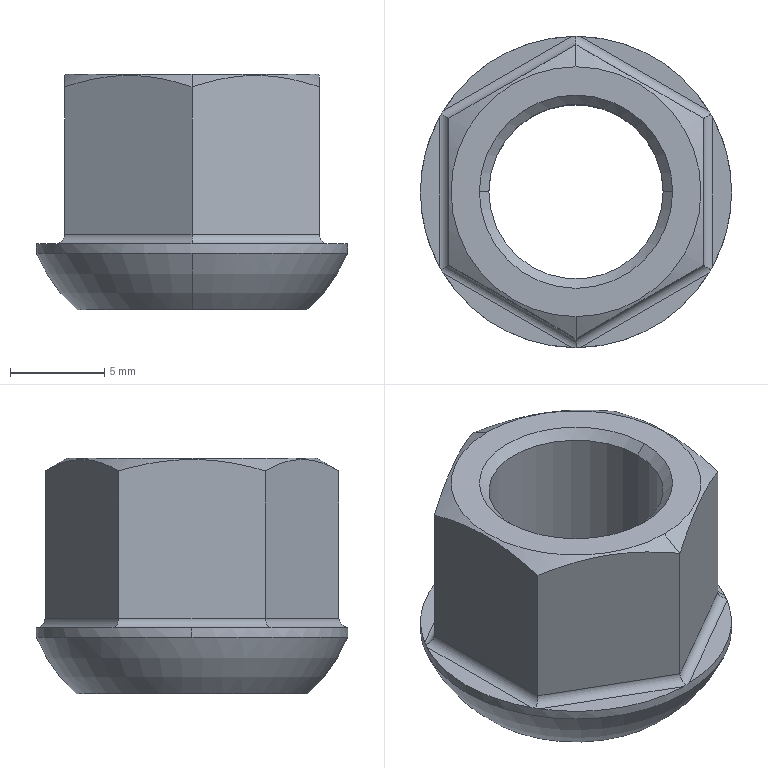Part | SolidWorks | features Chamfer 2, Extrusion 1, Fillet 1, HoleWzd 1, ICE 1, RevCut 1, Revolution 1, Scale 1 | 1 solid | 32 faces | box 16.5 x 16.5 x 12.5 mm | volume 1193 mm3 | plane 14 | cylinder 10 | cone 6 | torus 2 | commonest cylinder face diameters 1 x6 9.25 x2 16.5 x2
STEP:
#1=CARTESIAN_POINT('',(4.625,0.,-3.));
#2=VERTEX_POINT('',#1);
#3=CARTESIAN_POINT('',(-4.625,0.,-3.));
#4=VERTEX_POINT('',#3);
#5=CARTESIAN_POINT('',(0.,0.,-3.));
#6=DIRECTION('',(0.,0.,-1.));
#7=DIRECTION('',(-1.,0.,0.));
#8=AXIS2_PLACEMENT_3D('',#5,#6,#7);
#9=CIRCLE('',#8,4.625);
#10=EDGE_CURVE('',#2,#4,#9,.T.);
#11=ORIENTED_EDGE('',*,*,#10,.F.);
#12=CARTESIAN_POINT('',(5.125,0.,-3.5));
#13=VERTEX_POINT('',#12);
#14=CARTESIAN_POINT('',(5.125,0.,-3.5));
#15=DIRECTION('',(0.7071,0.,-0.7071));
#16=VECTOR('',#15,1000.);
#17=LINE('',#14,#16);
#18=EDGE_CURVE('',#2,#13,#17,.T.);
#19=ORIENTED_EDGE('',*,*,#18,.T.);
#20=CARTESIAN_POINT('',(-5.125,0.,-3.5));
#21=VERTEX_POINT('',#20);
#22=CARTESIAN_POINT('',(0.,0.,-3.5));
#23=DIRECTION('',(0.,0.,1.));
#24=DIRECTION('',(0.,1.,0.));
#25=AXIS2_PLACEMENT_3D('',#22,#23,#24);
#26=CIRCLE('',#25,5.125);
#27=EDGE_CURVE('',#21,#13,#26,.T.);
#28=ORIENTED_EDGE('',*,*,#27,.F.);
#29=CARTESIAN_POINT('',(-5.125,0.,-3.5));
#30=DIRECTION('',(-0.7071,0.,-0.7071));
#31=VECTOR('',#30,1000.);
#32=LINE('',#29,#31);
#33=EDGE_CURVE('',#4,#21,#32,.T.);
#34=ORIENTED_EDGE('',*,*,#33,.F.);
#35=EDGE_LOOP('',(#11,#19,#28,#34));
#36=FACE_OUTER_BOUND('',#35,.T.);
#37=CARTESIAN_POINT('',(0.,0.,-3.5));
#38=DIRECTION('',(0.,0.,-1.));
#39=DIRECTION('',(-1.,0.,0.));
#40=AXIS2_PLACEMENT_3D('',#37,#38,#39);
#41=CONICAL_SURFACE('',#40,5.125,0.7854);
#42=ADVANCED_FACE('',(#36),#41,.F.);
#43=CARTESIAN_POINT('',(-4.625,0.,8.5));
#44=VERTEX_POINT('',#43);
#45=CARTESIAN_POINT('',(4.625,0.,8.5));
#46=VERTEX_POINT('',#45);
#47=CARTESIAN_POINT('',(0.,0.,8.5));
#48=DIRECTION('',(0.,0.,1.));
#49=DIRECTION('',(1.,0.,0.));
#50=AXIS2_PLACEMENT_3D('',#47,#48,#49);
#51=CIRCLE('',#50,4.625);
#52=EDGE_CURVE('',#44,#46,#51,.T.);
#53=ORIENTED_EDGE('',*,*,#52,.F.);
#54=CARTESIAN_POINT('',(-5.125,0.,9.));
#55=VERTEX_POINT('',#54);
#56=CARTESIAN_POINT('',(-4.625,0.,8.5));
#57=DIRECTION('',(-0.7071,0.,0.7071));
#58=VECTOR('',#57,1000.);
#59=LINE('',#56,#58);
#60=EDGE_CURVE('',#44,#55,#59,.T.);
#61=ORIENTED_EDGE('',*,*,#60,.T.);
#62=CARTESIAN_POINT('',(5.125,0.,9.));
#63=VERTEX_POINT('',#62);
#64=CARTESIAN_POINT('',(0.,0.,9.));
#65=DIRECTION('',(0.,0.,-1.));
#66=DIRECTION('',(1.,0.,0.));
#67=AXIS2_PLACEMENT_3D('',#64,#65,#66);
#68=CIRCLE('',#67,5.125);
#69=EDGE_CURVE('',#63,#55,#68,.T.);
#70=ORIENTED_EDGE('',*,*,#69,.F.);
#71=CARTESIAN_POINT('',(4.625,0.,8.5));
#72=DIRECTION('',(0.7071,0.,0.7071));
#73=VECTOR('',#72,1000.);
#74=LINE('',#71,#73);
#75=EDGE_CURVE('',#46,#63,#74,.T.);
#76=ORIENTED_EDGE('',*,*,#75,.F.);
#77=EDGE_LOOP('',(#53,#61,#70,#76));
#78=FACE_OUTER_BOUND('',#77,.T.);
#79=CARTESIAN_POINT('',(0.,0.,8.5));
#80=DIRECTION('',(0.,0.,1.));
#81=DIRECTION('',(1.,0.,0.));
#82=AXIS2_PLACEMENT_3D('',#79,#80,#81);
#83=CONICAL_SURFACE('',#82,4.625,0.7854);
#84=ADVANCED_FACE('',(#78),#83,.F.);
#85=ORIENTED_EDGE('',*,*,#10,.T.);
#86=CARTESIAN_POINT('',(-4.625,0.,9.));
#87=DIRECTION('',(0.,0.,1.));
#88=VECTOR('',#87,1000.);
#89=LINE('',#86,#88);
#90=EDGE_CURVE('',#4,#44,#89,.T.);
#91=ORIENTED_EDGE('',*,*,#90,.T.);
#92=ORIENTED_EDGE('',*,*,#52,.T.);
#93=CARTESIAN_POINT('',(4.625,0.,9.));
#94=DIRECTION('',(0.,0.,1.));
#95=VECTOR('',#94,1000.);
#96=LINE('',#93,#95);
#97=EDGE_CURVE('',#2,#46,#96,.T.);
#98=ORIENTED_EDGE('',*,*,#97,.F.);
#99=EDGE_LOOP('',(#85,#91,#92,#98));
#100=FACE_OUTER_BOUND('',#99,.T.);
#101=CARTESIAN_POINT('',(0.,0.,9.));
#102=DIRECTION('',(0.,0.,1.));
#103=DIRECTION('',(1.,0.,0.));
#104=AXIS2_PLACEMENT_3D('',#101,#102,#103);
#105=CYLINDRICAL_SURFACE('',#104,4.625);
#106=ADVANCED_FACE('',(#100),#105,.F.);
#107=CARTESIAN_POINT('',(0.,6.625,9.));
#108=VERTEX_POINT('',#107);
#109=CARTESIAN_POINT('',(0.,-6.625,9.));
#110=VERTEX_POINT('',#109);
#111=CARTESIAN_POINT('',(0.,0.,9.));
#112=DIRECTION('',(0.,0.,-1.));
#113=DIRECTION('',(0.,1.,0.));
#114=AXIS2_PLACEMENT_3D('',#111,#112,#113);
#115=CIRCLE('',#114,6.625);
#116=EDGE_CURVE('',#108,#110,#115,.T.);
#117=ORIENTED_EDGE('',*,*,#116,.T.);
#118=CARTESIAN_POINT('',(0.,-7.794,8.325));
#119=VERTEX_POINT('',#118);
#120=CARTESIAN_POINT('',(0.,-6.625,9.));
#121=DIRECTION('',(0.,-0.866,-0.5));
#122=VECTOR('',#121,1000.);
#123=LINE('',#120,#122);
#124=EDGE_CURVE('',#110,#119,#123,.T.);
#125=ORIENTED_EDGE('',*,*,#124,.T.);
#126=CARTESIAN_POINT('',(6.75,-3.897,8.325));
#127=VERTEX_POINT('',#126);
#128=CARTESIAN_POINT('',(6.75,-3.897,8.325));
#129=CARTESIAN_POINT('',(6.199,-4.215,8.509));
#130=CARTESIAN_POINT('',(5.644,-4.536,8.66));
#131=CARTESIAN_POINT('',(4.522,-5.183,8.87));
#132=CARTESIAN_POINT('',(3.955,-5.511,8.927));
#133=CARTESIAN_POINT('',(3.095,-6.008,8.928));
#134=CARTESIAN_POINT('',(2.806,-6.174,8.914));
#135=CARTESIAN_POINT('',(2.236,-6.503,8.859));
#136=CARTESIAN_POINT('',(1.953,-6.667,8.818));
#137=CARTESIAN_POINT('',(1.108,-7.154,8.661));
#138=CARTESIAN_POINT('',(0.5518,-7.476,8.509));
#139=CARTESIAN_POINT('',(0.,-7.794,8.325));
#140=B_SPLINE_CURVE_WITH_KNOTS('',3,(#128,#129,#130,#131,#132,#133,#134,#135,#136,#137,#138,#139),.UNSPECIFIED.,.F.,.F.,(4,2,2,2,2,4),(0.000000119,0.001968,0.003936,0.00492,0.005904,0.007872),.UNSPECIFIED.);
#141=EDGE_CURVE('',#127,#119,#140,.T.);
#142=ORIENTED_EDGE('',*,*,#141,.F.);
#143=CARTESIAN_POINT('',(6.75,3.897,8.325));
#144=VERTEX_POINT('',#143);
#145=CARTESIAN_POINT('',(6.75,3.897,8.325));
#146=CARTESIAN_POINT('',(6.75,3.267,8.507));
#147=CARTESIAN_POINT('',(6.75,2.629,8.658));
#148=CARTESIAN_POINT('',(6.75,1.328,8.87));
#149=CARTESIAN_POINT('',(6.75,0.6599,8.928));
#150=CARTESIAN_POINT('',(6.75,-0.6576,8.928));
#151=CARTESIAN_POINT('',(6.75,-1.312,8.871));
#152=CARTESIAN_POINT('',(6.75,-2.614,8.661));
#153=CARTESIAN_POINT('',(6.75,-3.263,8.508));
#154=CARTESIAN_POINT('',(6.75,-3.897,8.325));
#155=B_SPLINE_CURVE_WITH_KNOTS('',3,(#145,#146,#147,#148,#149,#150,#151,#152,#153,#154),.UNSPECIFIED.,.F.,.F.,(4,2,2,2,4),(0.002869,0.004835,0.006802,0.008769,0.01074),.UNSPECIFIED.);
#156=EDGE_CURVE('',#144,#127,#155,.T.);
#157=ORIENTED_EDGE('',*,*,#156,.F.);
#158=CARTESIAN_POINT('',(0.,7.794,8.325));
#159=VERTEX_POINT('',#158);
#160=CARTESIAN_POINT('',(0.,7.794,8.325));
#161=CARTESIAN_POINT('',(0.5511,7.476,8.509));
#162=CARTESIAN_POINT('',(1.106,7.156,8.66));
#163=CARTESIAN_POINT('',(2.228,6.508,8.87));
#164=CARTESIAN_POINT('',(2.795,6.181,8.927));
#165=CARTESIAN_POINT('',(3.655,5.684,8.928));
#166=CARTESIAN_POINT('',(3.944,5.517,8.914));
#167=CARTESIAN_POINT('',(4.514,5.188,8.859));
#168=CARTESIAN_POINT('',(4.797,5.025,8.818));
#169=CARTESIAN_POINT('',(5.642,4.537,8.661));
#170=CARTESIAN_POINT('',(6.198,4.216,8.509));
#171=CARTESIAN_POINT('',(6.75,3.897,8.325));
#172=B_SPLINE_CURVE_WITH_KNOTS('',3,(#160,#161,#162,#163,#164,#165,#166,#167,#168,#169,#170,#171),.UNSPECIFIED.,.F.,.F.,(4,2,2,2,2,4),(0.000000119,0.001968,0.003936,0.00492,0.005904,0.007872),.UNSPECIFIED.);
#173=EDGE_CURVE('',#159,#144,#172,.T.);
#174=ORIENTED_EDGE('',*,*,#173,.F.);
#175=CARTESIAN_POINT('',(0.,6.625,9.));
#176=DIRECTION('',(0.,0.866,-0.5));
#177=VECTOR('',#176,1000.);
#178=LINE('',#175,#177);
#179=EDGE_CURVE('',#108,#159,#178,.T.);
#180=ORIENTED_EDGE('',*,*,#179,.F.);
#181=EDGE_LOOP('',(#117,#125,#142,#157,#174,#180));
#182=FACE_OUTER_BOUND('',#181,.T.);
#183=CARTESIAN_POINT('',(0.,0.,9.));
#184=DIRECTION('',(0.,0.,-1.));
#185=DIRECTION('',(0.,1.,0.));
#186=AXIS2_PLACEMENT_3D('',#183,#184,#185);
#187=CONICAL_SURFACE('',#186,6.625,1.047);
#188=ADVANCED_FACE('',(#182),#187,.T.);
#189=CARTESIAN_POINT('',(8.25,0.,-0.5));
#190=VERTEX_POINT('',#189);
#191=CARTESIAN_POINT('',(0.,-8.25,-0.5));
#192=VERTEX_POINT('',#191);
#193=CARTESIAN_POINT('',(0.,0.,-0.5));
#194=DIRECTION('',(0.,0.,-1.));
#195=DIRECTION('',(-1.,0.,0.));
#196=AXIS2_PLACEMENT_3D('',#193,#194,#195);
#197=CIRCLE('',#196,8.25);
#198=EDGE_CURVE('',#190,#192,#197,.T.);
#199=ORIENTED_EDGE('',*,*,#198,.T.);
#200=CARTESIAN_POINT('',(0.,-6.125,-3.5));
#201=VERTEX_POINT('',#200);
#202=CARTESIAN_POINT('',(0.,-0.834,2.5));
#203=DIRECTION('',(1.,0.,0.));
#204=DIRECTION('',(0.,1.,0.));
#205=AXIS2_PLACEMENT_3D('',#202,#203,#204);
#206=CIRCLE('',#205,8.);
#207=EDGE_CURVE('',#192,#201,#206,.T.);
#208=ORIENTED_EDGE('',*,*,#207,.T.);
#209=CARTESIAN_POINT('',(0.,6.125,-3.5));
#210=VERTEX_POINT('',#209);
#211=CARTESIAN_POINT('',(0.,0.,-3.5));
#212=DIRECTION('',(0.,0.,-1.));
#213=DIRECTION('',(0.,1.,0.));
#214=AXIS2_PLACEMENT_3D('',#211,#212,#213);
#215=CIRCLE('',#214,6.125);
#216=EDGE_CURVE('',#210,#201,#215,.T.);
#217=ORIENTED_EDGE('',*,*,#216,.F.);
#218=CARTESIAN_POINT('',(0.,8.25,-0.5));
#219=VERTEX_POINT('',#218);
#220=CARTESIAN_POINT('',(0.,0.834,2.5));
#221=DIRECTION('',(-1.,0.,0.));
#222=DIRECTION('',(0.,0.,1.));
#223=AXIS2_PLACEMENT_3D('',#220,#221,#222);
#224=CIRCLE('',#223,8.);
#225=EDGE_CURVE('',#219,#210,#224,.T.);
#226=ORIENTED_EDGE('',*,*,#225,.F.);
#227=CARTESIAN_POINT('',(0.,0.,-0.5));
#228=DIRECTION('',(0.,0.,-1.));
#229=DIRECTION('',(-1.,0.,0.));
#230=AXIS2_PLACEMENT_3D('',#227,#228,#229);
#231=CIRCLE('',#230,8.25);
#232=EDGE_CURVE('',#219,#190,#231,.T.);
#233=ORIENTED_EDGE('',*,*,#232,.T.);
#234=EDGE_LOOP('',(#199,#208,#217,#226,#233));
#235=FACE_OUTER_BOUND('',#234,.T.);
#236=CARTESIAN_POINT('',(0.,0.,2.5));
#237=DIRECTION('',(0.,0.,-1.));
#238=DIRECTION('',(0.,1.,0.));
#239=AXIS2_PLACEMENT_3D('',#236,#237,#238);
#240=TOROIDAL_SURFACE('',#239,0.834,8.);
#241=ADVANCED_FACE('',(#235),#240,.T.);
#242=CARTESIAN_POINT('',(-8.25,0.,-0.5));
#243=VERTEX_POINT('',#242);
#244=CARTESIAN_POINT('',(0.,0.,-0.5));
#245=DIRECTION('',(0.,0.,-1.));
#246=DIRECTION('',(-1.,0.,0.));
#247=AXIS2_PLACEMENT_3D('',#244,#245,#246);
#248=CIRCLE('',#247,8.25);
#249=EDGE_CURVE('',#243,#219,#248,.T.);
#250=ORIENTED_EDGE('',*,*,#249,.F.);
#251=CARTESIAN_POINT('',(-8.25,0.,0.));
#252=VERTEX_POINT('',#251);
#253=CARTESIAN_POINT('',(-8.25,0.,-0.5));
#254=DIRECTION('',(0.,0.,1.));
#255=VECTOR('',#254,1000.);
#256=LINE('',#253,#255);
#257=EDGE_CURVE('',#243,#252,#256,.T.);
#258=ORIENTED_EDGE('',*,*,#257,.T.);
#259=CARTESIAN_POINT('',(-7.25,3.937,0.));
#260=VERTEX_POINT('',#259);
#261=CARTESIAN_POINT('',(0.,0.,0.));
#262=DIRECTION('',(0.,0.,-1.));
#263=DIRECTION('',(-1.,0.,0.));
#264=AXIS2_PLACEMENT_3D('',#261,#262,#263);
#265=CIRCLE('',#264,8.25);
#266=EDGE_CURVE('',#252,#260,#265,.T.);
#267=ORIENTED_EDGE('',*,*,#266,.T.);
#268=CARTESIAN_POINT('',(-7.145,4.125,0.01121));
#269=VERTEX_POINT('',#268);
#270=CARTESIAN_POINT('',(-7.25,3.937,0.));
#271=CARTESIAN_POINT('',(-7.216,4.,0.));
#272=CARTESIAN_POINT('',(-7.181,4.063,0.003498));
#273=CARTESIAN_POINT('',(-7.145,4.125,0.01121));
#274=B_SPLINE_CURVE_WITH_KNOTS('',3,(#270,#271,#272,#273),.UNSPECIFIED.,.F.,.F.,(4,4),(0.,0.0002158),.UNSPECIFIED.);
#275=EDGE_CURVE('',#260,#269,#274,.T.);
#276=ORIENTED_EDGE('',*,*,#275,.T.);
#277=CARTESIAN_POINT('',(-7.035,4.31,0.));
#278=VERTEX_POINT('',#277);
#279=CARTESIAN_POINT('',(-7.145,4.125,0.01121));
#280=CARTESIAN_POINT('',(-7.109,4.187,0.003498));
#281=CARTESIAN_POINT('',(-7.072,4.249,0.));
#282=CARTESIAN_POINT('',(-7.035,4.31,0.));
#283=B_SPLINE_CURVE_WITH_KNOTS('',3,(#279,#280,#281,#282),.UNSPECIFIED.,.F.,.F.,(4,4),(0.,0.0002158),.UNSPECIFIED.);
#284=EDGE_CURVE('',#269,#278,#283,.T.);
#285=ORIENTED_EDGE('',*,*,#284,.T.);
#286=CARTESIAN_POINT('',(-0.2155,8.247,0.));
#287=VERTEX_POINT('',#286);
#288=CARTESIAN_POINT('',(0.,0.,0.));
#289=DIRECTION('',(0.,0.,-1.));
#290=DIRECTION('',(-1.,0.,0.));
#291=AXIS2_PLACEMENT_3D('',#288,#289,#290);
#292=CIRCLE('',#291,8.25);
#293=EDGE_CURVE('',#278,#287,#292,.T.);
#294=ORIENTED_EDGE('',*,*,#293,.T.);
#295=CARTESIAN_POINT('',(0.,8.25,0.01121));
#296=VERTEX_POINT('',#295);
#297=CARTESIAN_POINT('',(-0.2155,8.247,0.));
#298=CARTESIAN_POINT('',(-0.1435,8.249,0.));
#299=CARTESIAN_POINT('',(-0.07162,8.25,0.003498));
#300=CARTESIAN_POINT('',(0.,8.25,0.01121));
#301=B_SPLINE_CURVE_WITH_KNOTS('',3,(#297,#298,#299,#300),.UNSPECIFIED.,.F.,.F.,(4,4),(0.,0.0002158),.UNSPECIFIED.);
#302=EDGE_CURVE('',#287,#296,#301,.T.);
#303=ORIENTED_EDGE('',*,*,#302,.T.);
#304=CARTESIAN_POINT('',(0.2155,8.247,0.));
#305=VERTEX_POINT('',#304);
#306=CARTESIAN_POINT('',(0.,8.25,0.01121));
#307=CARTESIAN_POINT('',(0.07162,8.25,0.003498));
#308=CARTESIAN_POINT('',(0.1435,8.249,0.));
#309=CARTESIAN_POINT('',(0.2155,8.247,0.));
#310=B_SPLINE_CURVE_WITH_KNOTS('',3,(#306,#307,#308,#309),.UNSPECIFIED.,.F.,.F.,(4,4),(0.,0.0002158),.UNSPECIFIED.);
#311=EDGE_CURVE('',#296,#305,#310,.T.);
#312=ORIENTED_EDGE('',*,*,#311,.T.);
#313=CARTESIAN_POINT('',(7.035,4.31,0.));
#314=VERTEX_POINT('',#313);
#315=CARTESIAN_POINT('',(0.,0.,0.));
#316=DIRECTION('',(0.,0.,-1.));
#317=DIRECTION('',(-1.,0.,0.));
#318=AXIS2_PLACEMENT_3D('',#315,#316,#317);
#319=CIRCLE('',#318,8.25);
#320=EDGE_CURVE('',#305,#314,#319,.T.);
#321=ORIENTED_EDGE('',*,*,#320,.T.);
#322=CARTESIAN_POINT('',(7.145,4.125,0.01121));
#323=VERTEX_POINT('',#322);
#324=CARTESIAN_POINT('',(7.035,4.31,0.));
#325=CARTESIAN_POINT('',(7.072,4.249,0.));
#326=CARTESIAN_POINT('',(7.109,4.187,0.003498));
#327=CARTESIAN_POINT('',(7.145,4.125,0.01121));
#328=B_SPLINE_CURVE_WITH_KNOTS('',3,(#324,#325,#326,#327),.UNSPECIFIED.,.F.,.F.,(4,4),(0.,0.0002158),.UNSPECIFIED.);
#329=EDGE_CURVE('',#314,#323,#328,.T.);
#330=ORIENTED_EDGE('',*,*,#329,.T.);
#331=CARTESIAN_POINT('',(7.25,3.937,0.));
#332=VERTEX_POINT('',#331);
#333=CARTESIAN_POINT('',(7.145,4.125,0.01121));
#334=CARTESIAN_POINT('',(7.181,4.063,0.003498));
#335=CARTESIAN_POINT('',(7.216,4.,0.));
#336=CARTESIAN_POINT('',(7.25,3.937,0.));
#337=B_SPLINE_CURVE_WITH_KNOTS('',3,(#333,#334,#335,#336),.UNSPECIFIED.,.F.,.F.,(4,4),(0.,0.0002158),.UNSPECIFIED.);
#338=EDGE_CURVE('',#323,#332,#337,.T.);
#339=ORIENTED_EDGE('',*,*,#338,.T.);
#340=CARTESIAN_POINT('',(8.25,0.,0.));
#341=VERTEX_POINT('',#340);
#342=CARTESIAN_POINT('',(0.,0.,0.));
#343=DIRECTION('',(0.,0.,-1.));
#344=DIRECTION('',(-1.,0.,0.));
#345=AXIS2_PLACEMENT_3D('',#342,#343,#344);
#346=CIRCLE('',#345,8.25);
#347=EDGE_CURVE('',#332,#341,#346,.T.);
#348=ORIENTED_EDGE('',*,*,#347,.T.);
#349=CARTESIAN_POINT('',(8.25,0.,-0.5));
#350=DIRECTION('',(0.,0.,1.));
#351=VECTOR('',#350,1000.);
#352=LINE('',#349,#351);
#353=EDGE_CURVE('',#190,#341,#352,.T.);
#354=ORIENTED_EDGE('',*,*,#353,.F.);
#355=ORIENTED_EDGE('',*,*,#232,.F.);
#356=EDGE_LOOP('',(#250,#258,#267,#276,#285,#294,#303,#312,#321,#330,#339,#348,#354,#355));
#357=FACE_OUTER_BOUND('',#356,.T.);
#358=CARTESIAN_POINT('',(0.,0.,-0.5));
#359=DIRECTION('',(0.,0.,1.));
#360=DIRECTION('',(1.,0.,0.));
#361=AXIS2_PLACEMENT_3D('',#358,#359,#360);
#362=CYLINDRICAL_SURFACE('',#361,8.25);
#363=ADVANCED_FACE('',(#357),#362,.T.);
#364=ORIENTED_EDGE('',*,*,#293,.F.);
#365=CARTESIAN_POINT('',(-0.25,8.227,0.));
#366=DIRECTION('',(0.866,0.5,0.));
#367=VECTOR('',#366,1000.);
#368=LINE('',#365,#367);
#369=EDGE_CURVE('',#278,#287,#368,.T.);
#370=ORIENTED_EDGE('',*,*,#369,.T.);
#371=EDGE_LOOP('',(#364,#370));
#372=FACE_OUTER_BOUND('',#371,.T.);
#373=CARTESIAN_POINT('',(0.,0.,0.));
#374=DIRECTION('',(0.,0.,-1.));
#375=DIRECTION('',(-1.,0.,0.));
#376=AXIS2_PLACEMENT_3D('',#373,#374,#375);
#377=PLANE('',#376);
#378=ADVANCED_FACE('',(#372),#377,.F.);
#379=CARTESIAN_POINT('',(-7.25,-3.937,0.));
#380=VERTEX_POINT('',#379);
#381=CARTESIAN_POINT('',(0.,0.,0.));
#382=DIRECTION('',(0.,0.,-1.));
#383=DIRECTION('',(-1.,0.,0.));
#384=AXIS2_PLACEMENT_3D('',#381,#382,#383);
#385=CIRCLE('',#384,8.25);
#386=EDGE_CURVE('',#380,#252,#385,.T.);
#387=ORIENTED_EDGE('',*,*,#386,.F.);
#388=CARTESIAN_POINT('',(-7.25,3.897,0.));
#389=DIRECTION('',(0.,1.,0.));
#390=VECTOR('',#389,1000.);
#391=LINE('',#388,#390);
#392=EDGE_CURVE('',#380,#260,#391,.T.);
#393=ORIENTED_EDGE('',*,*,#392,.T.);
#394=ORIENTED_EDGE('',*,*,#266,.F.);
#395=EDGE_LOOP('',(#387,#393,#394));
#396=FACE_OUTER_BOUND('',#395,.T.);
#397=CARTESIAN_POINT('',(0.,0.,0.));
#398=DIRECTION('',(0.,0.,-1.));
#399=DIRECTION('',(-1.,0.,0.));
#400=AXIS2_PLACEMENT_3D('',#397,#398,#399);
#401=PLANE('',#400);
#402=ADVANCED_FACE('',(#396),#401,.F.);
#403=CARTESIAN_POINT('',(-0.2155,-8.247,0.));
#404=VERTEX_POINT('',#403);
#405=CARTESIAN_POINT('',(-7.035,-4.31,0.));
#406=VERTEX_POINT('',#405);
#407=CARTESIAN_POINT('',(0.,0.,0.));
#408=DIRECTION('',(0.,0.,-1.));
#409=DIRECTION('',(-1.,0.,0.));
#410=AXIS2_PLACEMENT_3D('',#407,#408,#409);
#411=CIRCLE('',#410,8.25);
#412=EDGE_CURVE('',#404,#406,#411,.T.);
#413=ORIENTED_EDGE('',*,*,#412,.F.);
#414=CARTESIAN_POINT('',(-7.,-4.33,0.));
#415=DIRECTION('',(-0.866,0.5,0.));
#416=VECTOR('',#415,1000.);
#417=LINE('',#414,#416);
#418=EDGE_CURVE('',#404,#406,#417,.T.);
#419=ORIENTED_EDGE('',*,*,#418,.T.);
#420=EDGE_LOOP('',(#413,#419));
#421=FACE_OUTER_BOUND('',#420,.T.);
#422=CARTESIAN_POINT('',(0.,0.,0.));
#423=DIRECTION('',(0.,0.,-1.));
#424=DIRECTION('',(-1.,0.,0.));
#425=AXIS2_PLACEMENT_3D('',#422,#423,#424);
#426=PLANE('',#425);
#427=ADVANCED_FACE('',(#421),#426,.F.);
#428=CARTESIAN_POINT('',(7.035,-4.31,0.));
#429=VERTEX_POINT('',#428);
#430=CARTESIAN_POINT('',(0.2155,-8.247,0.));
#431=VERTEX_POINT('',#430);
#432=CARTESIAN_POINT('',(0.,0.,0.));
#433=DIRECTION('',(0.,0.,-1.));
#434=DIRECTION('',(-1.,0.,0.));
#435=AXIS2_PLACEMENT_3D('',#432,#433,#434);
#436=CIRCLE('',#435,8.25);
#437=EDGE_CURVE('',#429,#431,#436,.T.);
#438=ORIENTED_EDGE('',*,*,#437,.F.);
#439=CARTESIAN_POINT('',(0.25,-8.227,0.));
#440=DIRECTION('',(-0.866,-0.5,0.));
#441=VECTOR('',#440,1000.);
#442=LINE('',#439,#441);
#443=EDGE_CURVE('',#429,#431,#442,.T.);
#444=ORIENTED_EDGE('',*,*,#443,.T.);
#445=EDGE_LOOP('',(#438,#444));
#446=FACE_OUTER_BOUND('',#445,.T.);
#447=CARTESIAN_POINT('',(0.,0.,0.));
#448=DIRECTION('',(0.,0.,-1.));
#449=DIRECTION('',(-1.,0.,0.));
#450=AXIS2_PLACEMENT_3D('',#447,#448,#449);
#451=PLANE('',#450);
#452=ADVANCED_FACE('',(#446),#451,.F.);
#453=ORIENTED_EDGE('',*,*,#347,.F.);
#454=CARTESIAN_POINT('',(7.25,-3.937,0.));
#455=VERTEX_POINT('',#454);
#456=CARTESIAN_POINT('',(7.25,-3.897,0.));
#457=DIRECTION('',(0.,-1.,0.));
#458=VECTOR('',#457,1000.);
#459=LINE('',#456,#458);
#460=EDGE_CURVE('',#332,#455,#459,.T.);
#461=ORIENTED_EDGE('',*,*,#460,.T.);
#462=CARTESIAN_POINT('',(0.,0.,0.));
#463=DIRECTION('',(0.,0.,-1.));
#464=DIRECTION('',(-1.,0.,0.));
#465=AXIS2_PLACEMENT_3D('',#462,#463,#464);
#466=CIRCLE('',#465,8.25);
#467=EDGE_CURVE('',#341,#455,#466,.T.);
#468=ORIENTED_EDGE('',*,*,#467,.F.);
#469=EDGE_LOOP('',(#453,#461,#468));
#470=FACE_OUTER_BOUND('',#469,.T.);
#471=CARTESIAN_POINT('',(0.,0.,0.));
#472=DIRECTION('',(0.,0.,-1.));
#473=DIRECTION('',(-1.,0.,0.));
#474=AXIS2_PLACEMENT_3D('',#471,#472,#473);
#475=PLANE('',#474);
#476=ADVANCED_FACE('',(#470),#475,.F.);
#477=CARTESIAN_POINT('',(-6.75,-3.897,8.325));
#478=VERTEX_POINT('',#477);
#479=CARTESIAN_POINT('',(-6.75,-3.897,0.5));
#480=VERTEX_POINT('',#479);
#481=CARTESIAN_POINT('',(-6.75,-3.897,9.));
#482=DIRECTION('',(0.,0.,-1.));
#483=VECTOR('',#482,1000.);
#484=LINE('',#481,#483);
#485=EDGE_CURVE('',#478,#480,#484,.T.);
#486=ORIENTED_EDGE('',*,*,#485,.T.);
#487=CARTESIAN_POINT('',(0.,-7.794,0.5));
#488=VERTEX_POINT('',#487);
#489=CARTESIAN_POINT('',(0.,-7.794,0.5));
#490=DIRECTION('',(0.866,-0.5,0.));
#491=VECTOR('',#490,1000.);
#492=LINE('',#489,#491);
#493=EDGE_CURVE('',#480,#488,#492,.T.);
#494=ORIENTED_EDGE('',*,*,#493,.T.);
#495=CARTESIAN_POINT('',(0.,-7.794,9.));
#496=DIRECTION('',(0.,0.,-1.));
#497=VECTOR('',#496,1000.);
#498=LINE('',#495,#497);
#499=EDGE_CURVE('',#119,#488,#498,.T.);
#500=ORIENTED_EDGE('',*,*,#499,.F.);
#501=CARTESIAN_POINT('',(0.,-7.794,8.325));
#502=CARTESIAN_POINT('',(-0.5511,-7.476,8.509));
#503=CARTESIAN_POINT('',(-1.106,-7.156,8.66));
#504=CARTESIAN_POINT('',(-2.228,-6.508,8.87));
#505=CARTESIAN_POINT('',(-2.795,-6.181,8.927));
#506=CARTESIAN_POINT('',(-3.655,-5.684,8.928));
#507=CARTESIAN_POINT('',(-3.944,-5.517,8.914));
#508=CARTESIAN_POINT('',(-4.514,-5.188,8.859));
#509=CARTESIAN_POINT('',(-4.797,-5.025,8.818));
#510=CARTESIAN_POINT('',(-5.642,-4.537,8.661));
#511=CARTESIAN_POINT('',(-6.198,-4.216,8.509));
#512=CARTESIAN_POINT('',(-6.75,-3.897,8.325));
#513=B_SPLINE_CURVE_WITH_KNOTS('',3,(#501,#502,#503,#504,#505,#506,#507,#508,#509,#510,#511,#512),.UNSPECIFIED.,.F.,.F.,(4,2,2,2,2,4),(0.000000119,0.001968,0.003936,0.00492,0.005904,0.007872),.UNSPECIFIED.);
#514=EDGE_CURVE('',#119,#478,#513,.T.);
#515=ORIENTED_EDGE('',*,*,#514,.T.);
#516=EDGE_LOOP('',(#486,#494,#500,#515));
#517=FACE_OUTER_BOUND('',#516,.T.);
#518=CARTESIAN_POINT('',(-6.75,-3.897,9.));
#519=DIRECTION('',(0.5,0.866,0.));
#520=DIRECTION('',(-0.866,0.5,0.));
#521=AXIS2_PLACEMENT_3D('',#518,#519,#520);
#522=PLANE('',#521);
#523=ADVANCED_FACE('',(#517),#522,.F.);
#524=ORIENTED_EDGE('',*,*,#499,.T.);
#525=CARTESIAN_POINT('',(6.75,-3.897,0.5));
#526=VERTEX_POINT('',#525);
#527=CARTESIAN_POINT('',(6.75,-3.897,0.5));
#528=DIRECTION('',(0.866,0.5,0.));
#529=VECTOR('',#528,1000.);
#530=LINE('',#527,#529);
#531=EDGE_CURVE('',#488,#526,#530,.T.);
#532=ORIENTED_EDGE('',*,*,#531,.T.);
#533=CARTESIAN_POINT('',(6.75,-3.897,9.));
#534=DIRECTION('',(0.,0.,-1.));
#535=VECTOR('',#534,1000.);
#536=LINE('',#533,#535);
#537=EDGE_CURVE('',#127,#526,#536,.T.);
#538=ORIENTED_EDGE('',*,*,#537,.F.);
#539=ORIENTED_EDGE('',*,*,#141,.T.);
#540=EDGE_LOOP('',(#524,#532,#538,#539));
#541=FACE_OUTER_BOUND('',#540,.T.);
#542=CARTESIAN_POINT('',(0.,-7.794,9.));
#543=DIRECTION('',(-0.5,0.866,0.));
#544=DIRECTION('',(-0.866,-0.5,0.));
#545=AXIS2_PLACEMENT_3D('',#542,#543,#544);
#546=PLANE('',#545);
#547=ADVANCED_FACE('',(#541),#546,.F.);
#548=ORIENTED_EDGE('',*,*,#537,.T.);
#549=CARTESIAN_POINT('',(6.75,3.897,0.5));
#550=VERTEX_POINT('',#549);
#551=CARTESIAN_POINT('',(6.75,3.897,0.5));
#552=DIRECTION('',(0.,1.,0.));
#553=VECTOR('',#552,1000.);
#554=LINE('',#551,#553);
#555=EDGE_CURVE('',#526,#550,#554,.T.);
#556=ORIENTED_EDGE('',*,*,#555,.T.);
#557=CARTESIAN_POINT('',(6.75,3.897,9.));
#558=DIRECTION('',(0.,0.,-1.));
#559=VECTOR('',#558,1000.);
#560=LINE('',#557,#559);
#561=EDGE_CURVE('',#144,#550,#560,.T.);
#562=ORIENTED_EDGE('',*,*,#561,.F.);
#563=ORIENTED_EDGE('',*,*,#156,.T.);
#564=EDGE_LOOP('',(#548,#556,#562,#563));
#565=FACE_OUTER_BOUND('',#564,.T.);
#566=CARTESIAN_POINT('',(6.75,-3.897,9.));
#567=DIRECTION('',(-1.,0.,0.));
#568=DIRECTION('',(0.,-1.,0.));
#569=AXIS2_PLACEMENT_3D('',#566,#567,#568);
#570=PLANE('',#569);
#571=ADVANCED_FACE('',(#565),#570,.F.);
#572=ORIENTED_EDGE('',*,*,#561,.T.);
#573=CARTESIAN_POINT('',(0.,7.794,0.5));
#574=VERTEX_POINT('',#573);
#575=CARTESIAN_POINT('',(0.,7.794,0.5));
#576=DIRECTION('',(-0.866,0.5,0.));
#577=VECTOR('',#576,1000.);
#578=LINE('',#575,#577);
#579=EDGE_CURVE('',#550,#574,#578,.T.);
#580=ORIENTED_EDGE('',*,*,#579,.T.);
#581=CARTESIAN_POINT('',(0.,7.794,9.));
#582=DIRECTION('',(0.,0.,-1.));
#583=VECTOR('',#582,1000.);
#584=LINE('',#581,#583);
#585=EDGE_CURVE('',#159,#574,#584,.T.);
#586=ORIENTED_EDGE('',*,*,#585,.F.);
#587=ORIENTED_EDGE('',*,*,#173,.T.);
#588=EDGE_LOOP('',(#572,#580,#586,#587));
#589=FACE_OUTER_BOUND('',#588,.T.);
#590=CARTESIAN_POINT('',(6.75,3.897,9.));
#591=DIRECTION('',(-0.5,-0.866,0.));
#592=DIRECTION('',(0.866,-0.5,0.));
#593=AXIS2_PLACEMENT_3D('',#590,#591,#592);
#594=PLANE('',#593);
#595=ADVANCED_FACE('',(#589),#594,.F.);
#596=ORIENTED_EDGE('',*,*,#585,.T.);
#597=CARTESIAN_POINT('',(-6.75,3.897,0.5));
#598=VERTEX_POINT('',#597);
#599=CARTESIAN_POINT('',(-6.75,3.897,0.5));
#600=DIRECTION('',(-0.866,-0.5,0.));
#601=VECTOR('',#600,1000.);
#602=LINE('',#599,#601);
#603=EDGE_CURVE('',#574,#598,#602,.T.);
#604=ORIENTED_EDGE('',*,*,#603,.T.);
#605=CARTESIAN_POINT('',(-6.75,3.897,8.325));
#606=VERTEX_POINT('',#605);
#607=CARTESIAN_POINT('',(-6.75,3.897,9.));
#608=DIRECTION('',(0.,0.,-1.));
#609=VECTOR('',#608,1000.);
#610=LINE('',#607,#609);
#611=EDGE_CURVE('',#606,#598,#610,.T.);
#612=ORIENTED_EDGE('',*,*,#611,.F.);
#613=CARTESIAN_POINT('',(-6.75,3.897,8.325));
#614=CARTESIAN_POINT('',(-6.199,4.215,8.509));
#615=CARTESIAN_POINT('',(-5.644,4.536,8.66));
#616=CARTESIAN_POINT('',(-4.522,5.183,8.87));
#617=CARTESIAN_POINT('',(-3.955,5.511,8.927));
#618=CARTESIAN_POINT('',(-3.095,6.008,8.928));
#619=CARTESIAN_POINT('',(-2.806,6.174,8.914));
#620=CARTESIAN_POINT('',(-2.236,6.503,8.859));
#621=CARTESIAN_POINT('',(-1.953,6.667,8.818));
#622=CARTESIAN_POINT('',(-1.108,7.154,8.661));
#623=CARTESIAN_POINT('',(-0.5518,7.476,8.509));
#624=CARTESIAN_POINT('',(0.,7.794,8.325));
#625=B_SPLINE_CURVE_WITH_KNOTS('',3,(#613,#614,#615,#616,#617,#618,#619,#620,#621,#622,#623,#624),.UNSPECIFIED.,.F.,.F.,(4,2,2,2,2,4),(0.000000119,0.001968,0.003936,0.00492,0.005904,0.007872),.UNSPECIFIED.);
#626=EDGE_CURVE('',#606,#159,#625,.T.);
#627=ORIENTED_EDGE('',*,*,#626,.T.);
#628=EDGE_LOOP('',(#596,#604,#612,#627));
#629=FACE_OUTER_BOUND('',#628,.T.);
#630=CARTESIAN_POINT('',(0.,7.794,9.));
#631=DIRECTION('',(0.5,-0.866,0.));
#632=DIRECTION('',(0.866,0.5,0.));
#633=AXIS2_PLACEMENT_3D('',#630,#631,#632);
#634=PLANE('',#633);
#635=ADVANCED_FACE('',(#629),#634,.F.);
#636=ORIENTED_EDGE('',*,*,#611,.T.);
#637=CARTESIAN_POINT('',(-6.75,-3.897,0.5));
#638=DIRECTION('',(0.,-1.,0.));
#639=VECTOR('',#638,1000.);
#640=LINE('',#637,#639);
#641=EDGE_CURVE('',#598,#480,#640,.T.);
#642=ORIENTED_EDGE('',*,*,#641,.T.);
#643=ORIENTED_EDGE('',*,*,#485,.F.);
#644=CARTESIAN_POINT('',(-6.75,-3.897,8.325));
#645=CARTESIAN_POINT('',(-6.75,-3.263,8.508));
#646=CARTESIAN_POINT('',(-6.75,-2.614,8.661));
#647=CARTESIAN_POINT('',(-6.75,-1.312,8.871));
#648=CARTESIAN_POINT('',(-6.75,-0.6576,8.928));
#649=CARTESIAN_POINT('',(-6.75,0.6599,8.928));
#650=CARTESIAN_POINT('',(-6.75,1.328,8.87));
#651=CARTESIAN_POINT('',(-6.75,2.629,8.658));
#652=CARTESIAN_POINT('',(-6.75,3.267,8.507));
#653=CARTESIAN_POINT('',(-6.75,3.897,8.325));
#654=B_SPLINE_CURVE_WITH_KNOTS('',3,(#644,#645,#646,#647,#648,#649,#650,#651,#652,#653),.UNSPECIFIED.,.F.,.F.,(4,2,2,2,4),(0.006942,0.008914,0.01089,0.01286,0.01483),.UNSPECIFIED.);
#655=EDGE_CURVE('',#478,#606,#654,.T.);
#656=ORIENTED_EDGE('',*,*,#655,.T.);
#657=EDGE_LOOP('',(#636,#642,#643,#656));
#658=FACE_OUTER_BOUND('',#657,.T.);
#659=CARTESIAN_POINT('',(-6.75,3.897,9.));
#660=DIRECTION('',(1.,0.,0.));
#661=DIRECTION('',(0.,1.,0.));
#662=AXIS2_PLACEMENT_3D('',#659,#660,#661);
#663=PLANE('',#662);
#664=ADVANCED_FACE('',(#658),#663,.F.);
#665=ORIENTED_EDGE('',*,*,#320,.F.);
#666=CARTESIAN_POINT('',(7.,4.33,0.));
#667=DIRECTION('',(0.866,-0.5,0.));
#668=VECTOR('',#667,1000.);
#669=LINE('',#666,#668);
#670=EDGE_CURVE('',#305,#314,#669,.T.);
#671=ORIENTED_EDGE('',*,*,#670,.T.);
#672=EDGE_LOOP('',(#665,#671));
#673=FACE_OUTER_BOUND('',#672,.T.);
#674=CARTESIAN_POINT('',(0.,0.,0.));
#675=DIRECTION('',(0.,0.,-1.));
#676=DIRECTION('',(-1.,0.,0.));
#677=AXIS2_PLACEMENT_3D('',#674,#675,#676);
#678=PLANE('',#677);
#679=ADVANCED_FACE('',(#673),#678,.F.);
#680=ORIENTED_EDGE('',*,*,#257,.F.);
#681=CARTESIAN_POINT('',(0.,0.,-0.5));
#682=DIRECTION('',(0.,0.,-1.));
#683=DIRECTION('',(-1.,0.,0.));
#684=AXIS2_PLACEMENT_3D('',#681,#682,#683);
#685=CIRCLE('',#684,8.25);
#686=EDGE_CURVE('',#192,#243,#685,.T.);
#687=ORIENTED_EDGE('',*,*,#686,.F.);
#688=ORIENTED_EDGE('',*,*,#198,.F.);
#689=ORIENTED_EDGE('',*,*,#353,.T.);
#690=ORIENTED_EDGE('',*,*,#467,.T.);
#691=CARTESIAN_POINT('',(7.145,-4.125,0.01121));
#692=VERTEX_POINT('',#691);
#693=CARTESIAN_POINT('',(7.25,-3.937,0.));
#694=CARTESIAN_POINT('',(7.216,-4.,0.));
#695=CARTESIAN_POINT('',(7.181,-4.063,0.003498));
#696=CARTESIAN_POINT('',(7.145,-4.125,0.01121));
#697=B_SPLINE_CURVE_WITH_KNOTS('',3,(#693,#694,#695,#696),.UNSPECIFIED.,.F.,.F.,(4,4),(0.,0.0002158),.UNSPECIFIED.);
#698=EDGE_CURVE('',#455,#692,#697,.T.);
#699=ORIENTED_EDGE('',*,*,#698,.T.);
#700=CARTESIAN_POINT('',(7.145,-4.125,0.01121));
#701=CARTESIAN_POINT('',(7.109,-4.187,0.003498));
#702=CARTESIAN_POINT('',(7.072,-4.249,0.));
#703=CARTESIAN_POINT('',(7.035,-4.31,0.));
#704=B_SPLINE_CURVE_WITH_KNOTS('',3,(#700,#701,#702,#703),.UNSPECIFIED.,.F.,.F.,(4,4),(0.,0.0002158),.UNSPECIFIED.);
#705=EDGE_CURVE('',#692,#429,#704,.T.);
#706=ORIENTED_EDGE('',*,*,#705,.T.);
#707=ORIENTED_EDGE('',*,*,#437,.T.);
#708=CARTESIAN_POINT('',(0.,-8.25,0.01121));
#709=VERTEX_POINT('',#708);
#710=CARTESIAN_POINT('',(0.2155,-8.247,0.));
#711=CARTESIAN_POINT('',(0.1435,-8.249,0.));
#712=CARTESIAN_POINT('',(0.07162,-8.25,0.003498));
#713=CARTESIAN_POINT('',(0.,-8.25,0.01121));
#714=B_SPLINE_CURVE_WITH_KNOTS('',3,(#710,#711,#712,#713),.UNSPECIFIED.,.F.,.F.,(4,4),(0.,0.0002158),.UNSPECIFIED.);
#715=EDGE_CURVE('',#431,#709,#714,.T.);
#716=ORIENTED_EDGE('',*,*,#715,.T.);
#717=CARTESIAN_POINT('',(0.,-8.25,0.01121));
#718=CARTESIAN_POINT('',(-0.07162,-8.25,0.003498));
#719=CARTESIAN_POINT('',(-0.1435,-8.249,0.));
#720=CARTESIAN_POINT('',(-0.2155,-8.247,0.));
#721=B_SPLINE_CURVE_WITH_KNOTS('',3,(#717,#718,#719,#720),.UNSPECIFIED.,.F.,.F.,(4,4),(0.,0.0002158),.UNSPECIFIED.);
#722=EDGE_CURVE('',#709,#404,#721,.T.);
#723=ORIENTED_EDGE('',*,*,#722,.T.);
#724=ORIENTED_EDGE('',*,*,#412,.T.);
#725=CARTESIAN_POINT('',(-7.145,-4.125,0.01121));
#726=VERTEX_POINT('',#725);
#727=CARTESIAN_POINT('',(-7.035,-4.31,0.));
#728=CARTESIAN_POINT('',(-7.072,-4.249,0.));
#729=CARTESIAN_POINT('',(-7.109,-4.187,0.003498));
#730=CARTESIAN_POINT('',(-7.145,-4.125,0.01121));
#731=B_SPLINE_CURVE_WITH_KNOTS('',3,(#727,#728,#729,#730),.UNSPECIFIED.,.F.,.F.,(4,4),(0.,0.0002158),.UNSPECIFIED.);
#732=EDGE_CURVE('',#406,#726,#731,.T.);
#733=ORIENTED_EDGE('',*,*,#732,.T.);
#734=CARTESIAN_POINT('',(-7.145,-4.125,0.01121));
#735=CARTESIAN_POINT('',(-7.181,-4.063,0.003498));
#736=CARTESIAN_POINT('',(-7.216,-4.,0.));
#737=CARTESIAN_POINT('',(-7.25,-3.937,0.));
#738=B_SPLINE_CURVE_WITH_KNOTS('',3,(#734,#735,#736,#737),.UNSPECIFIED.,.F.,.F.,(4,4),(0.,0.0002158),.UNSPECIFIED.);
#739=EDGE_CURVE('',#726,#380,#738,.T.);
#740=ORIENTED_EDGE('',*,*,#739,.T.);
#741=ORIENTED_EDGE('',*,*,#386,.T.);
#742=EDGE_LOOP('',(#680,#687,#688,#689,#690,#699,#706,#707,#716,#723,#724,#733,#740,#741));
#743=FACE_OUTER_BOUND('',#742,.T.);
#744=CARTESIAN_POINT('',(0.,0.,-0.5));
#745=DIRECTION('',(0.,0.,1.));
#746=DIRECTION('',(1.,0.,0.));
#747=AXIS2_PLACEMENT_3D('',#744,#745,#746);
#748=CYLINDRICAL_SURFACE('',#747,8.25);
#749=ADVANCED_FACE('',(#743),#748,.T.);
#750=ORIENTED_EDGE('',*,*,#27,.T.);
#751=CARTESIAN_POINT('',(0.,0.,-3.5));
#752=DIRECTION('',(0.,0.,1.));
#753=DIRECTION('',(0.,1.,0.));
#754=AXIS2_PLACEMENT_3D('',#751,#752,#753);
#755=CIRCLE('',#754,5.125);
#756=EDGE_CURVE('',#13,#21,#755,.T.);
#757=ORIENTED_EDGE('',*,*,#756,.T.);
#758=EDGE_LOOP('',(#750,#757));
#759=FACE_BOUND('',#758,.T.);
#760=ORIENTED_EDGE('',*,*,#216,.T.);
#761=CARTESIAN_POINT('',(0.,0.,-3.5));
#762=DIRECTION('',(0.,0.,-1.));
#763=DIRECTION('',(0.,1.,0.));
#764=AXIS2_PLACEMENT_3D('',#761,#762,#763);
#765=CIRCLE('',#764,6.125);
#766=EDGE_CURVE('',#201,#210,#765,.T.);
#767=ORIENTED_EDGE('',*,*,#766,.T.);
#768=EDGE_LOOP('',(#760,#767));
#769=FACE_OUTER_BOUND('',#768,.T.);
#770=CARTESIAN_POINT('',(0.,0.,-3.5));
#771=DIRECTION('',(0.,0.,-1.));
#772=DIRECTION('',(0.,1.,0.));
#773=AXIS2_PLACEMENT_3D('',#770,#771,#772);
#774=PLANE('',#773);
#775=ADVANCED_FACE('',(#759,#769),#774,.T.);
#776=ORIENTED_EDGE('',*,*,#207,.F.);
#777=ORIENTED_EDGE('',*,*,#686,.T.);
#778=ORIENTED_EDGE('',*,*,#249,.T.);
#779=ORIENTED_EDGE('',*,*,#225,.T.);
#780=ORIENTED_EDGE('',*,*,#766,.F.);
#781=EDGE_LOOP('',(#776,#777,#778,#779,#780));
#782=FACE_OUTER_BOUND('',#781,.T.);
#783=CARTESIAN_POINT('',(0.,0.,2.5));
#784=DIRECTION('',(0.,0.,-1.));
#785=DIRECTION('',(0.,1.,0.));
#786=AXIS2_PLACEMENT_3D('',#783,#784,#785);
#787=TOROIDAL_SURFACE('',#786,0.834,8.);
#788=ADVANCED_FACE('',(#782),#787,.T.);
#789=ORIENTED_EDGE('',*,*,#124,.F.);
#790=CARTESIAN_POINT('',(0.,0.,9.));
#791=DIRECTION('',(0.,0.,-1.));
#792=DIRECTION('',(0.,1.,0.));
#793=AXIS2_PLACEMENT_3D('',#790,#791,#792);
#794=CIRCLE('',#793,6.625);
#795=EDGE_CURVE('',#110,#108,#794,.T.);
#796=ORIENTED_EDGE('',*,*,#795,.T.);
#797=ORIENTED_EDGE('',*,*,#179,.T.);
#798=ORIENTED_EDGE('',*,*,#626,.F.);
#799=ORIENTED_EDGE('',*,*,#655,.F.);
#800=ORIENTED_EDGE('',*,*,#514,.F.);
#801=EDGE_LOOP('',(#789,#796,#797,#798,#799,#800));
#802=FACE_OUTER_BOUND('',#801,.T.);
#803=CARTESIAN_POINT('',(0.,0.,9.));
#804=DIRECTION('',(0.,0.,-1.));
#805=DIRECTION('',(0.,1.,0.));
#806=AXIS2_PLACEMENT_3D('',#803,#804,#805);
#807=CONICAL_SURFACE('',#806,6.625,1.047);
#808=ADVANCED_FACE('',(#802),#807,.T.);
#809=ORIENTED_EDGE('',*,*,#69,.T.);
#810=CARTESIAN_POINT('',(0.,0.,9.));
#811=DIRECTION('',(0.,0.,-1.));
#812=DIRECTION('',(1.,0.,0.));
#813=AXIS2_PLACEMENT_3D('',#810,#811,#812);
#814=CIRCLE('',#813,5.125);
#815=EDGE_CURVE('',#55,#63,#814,.T.);
#816=ORIENTED_EDGE('',*,*,#815,.T.);
#817=EDGE_LOOP('',(#809,#816));
#818=FACE_BOUND('',#817,.T.);
#819=ORIENTED_EDGE('',*,*,#116,.F.);
#820=ORIENTED_EDGE('',*,*,#795,.F.);
#821=EDGE_LOOP('',(#819,#820));
#822=FACE_OUTER_BOUND('',#821,.T.);
#823=CARTESIAN_POINT('',(0.,0.,9.));
#824=DIRECTION('',(0.,0.,1.));
#825=DIRECTION('',(1.,0.,0.));
#826=AXIS2_PLACEMENT_3D('',#823,#824,#825);
#827=PLANE('',#826);
#828=ADVANCED_FACE('',(#818,#822),#827,.T.);
#829=ORIENTED_EDGE('',*,*,#443,.F.);
#830=ORIENTED_EDGE('',*,*,#705,.F.);
#831=CARTESIAN_POINT('',(6.75,-3.897,0.5));
#832=CARTESIAN_POINT('',(6.75,-3.897,0.2542));
#833=CARTESIAN_POINT('',(6.904,-3.986,0.06297));
#834=CARTESIAN_POINT('',(7.145,-4.125,0.01121));
#835=(BOUNDED_CURVE()B_SPLINE_CURVE(3,(#831,#832,#833,#834),.UNSPECIFIED.,.F.,.T.)B_SPLINE_CURVE_WITH_KNOTS((4,4),(0.,1.359),.UNSPECIFIED.)CURVE()GEOMETRIC_REPRESENTATION_ITEM()RATIONAL_B_SPLINE_CURVE((1.,0.852,0.852,1.))REPRESENTATION_ITEM(''));
#836=EDGE_CURVE('',#526,#692,#835,.T.);
#837=ORIENTED_EDGE('',*,*,#836,.F.);
#838=ORIENTED_EDGE('',*,*,#531,.F.);
#839=CARTESIAN_POINT('',(0.,-8.25,0.01121));
#840=CARTESIAN_POINT('',(0.,-7.973,0.06297));
#841=CARTESIAN_POINT('',(0.,-7.794,0.2542));
#842=CARTESIAN_POINT('',(0.,-7.794,0.5));
#843=(BOUNDED_CURVE()B_SPLINE_CURVE(3,(#839,#840,#841,#842),.UNSPECIFIED.,.F.,.T.)B_SPLINE_CURVE_WITH_KNOTS((4,4),(4.925,6.283),.UNSPECIFIED.)CURVE()GEOMETRIC_REPRESENTATION_ITEM()RATIONAL_B_SPLINE_CURVE((1.,0.852,0.852,1.))REPRESENTATION_ITEM(''));
#844=EDGE_CURVE('',#709,#488,#843,.T.);
#845=ORIENTED_EDGE('',*,*,#844,.F.);
#846=ORIENTED_EDGE('',*,*,#715,.F.);
#847=EDGE_LOOP('',(#829,#830,#837,#838,#845,#846));
#848=FACE_OUTER_BOUND('',#847,.T.);
#849=CARTESIAN_POINT('',(0.25,-8.227,0.5));
#850=DIRECTION('',(-0.866,-0.5,0.));
#851=DIRECTION('',(0.5,-0.866,0.));
#852=AXIS2_PLACEMENT_3D('',#849,#850,#851);
#853=CYLINDRICAL_SURFACE('',#852,0.5);
#854=ADVANCED_FACE('',(#848),#853,.F.);
#855=ORIENTED_EDGE('',*,*,#460,.F.);
#856=ORIENTED_EDGE('',*,*,#338,.F.);
#857=CARTESIAN_POINT('',(6.75,3.897,0.5));
#858=CARTESIAN_POINT('',(6.75,3.897,0.2542));
#859=CARTESIAN_POINT('',(6.904,3.986,0.06297));
#860=CARTESIAN_POINT('',(7.145,4.125,0.01121));
#861=(BOUNDED_CURVE()B_SPLINE_CURVE(3,(#857,#858,#859,#860),.UNSPECIFIED.,.F.,.T.)B_SPLINE_CURVE_WITH_KNOTS((4,4),(0.,1.359),.UNSPECIFIED.)CURVE()GEOMETRIC_REPRESENTATION_ITEM()RATIONAL_B_SPLINE_CURVE((1.,0.852,0.852,1.))REPRESENTATION_ITEM(''));
#862=EDGE_CURVE('',#550,#323,#861,.T.);
#863=ORIENTED_EDGE('',*,*,#862,.F.);
#864=ORIENTED_EDGE('',*,*,#555,.F.);
#865=ORIENTED_EDGE('',*,*,#836,.T.);
#866=ORIENTED_EDGE('',*,*,#698,.F.);
#867=EDGE_LOOP('',(#855,#856,#863,#864,#865,#866));
#868=FACE_OUTER_BOUND('',#867,.T.);
#869=CARTESIAN_POINT('',(7.25,-3.897,0.5));
#870=DIRECTION('',(0.,-1.,0.));
#871=DIRECTION('',(1.,0.,0.));
#872=AXIS2_PLACEMENT_3D('',#869,#870,#871);
#873=CYLINDRICAL_SURFACE('',#872,0.5);
#874=ADVANCED_FACE('',(#868),#873,.F.);
#875=ORIENTED_EDGE('',*,*,#844,.T.);
#876=ORIENTED_EDGE('',*,*,#493,.F.);
#877=CARTESIAN_POINT('',(-7.145,-4.125,0.01121));
#878=CARTESIAN_POINT('',(-6.904,-3.986,0.06297));
#879=CARTESIAN_POINT('',(-6.75,-3.897,0.2542));
#880=CARTESIAN_POINT('',(-6.75,-3.897,0.5));
#881=(BOUNDED_CURVE()B_SPLINE_CURVE(3,(#877,#878,#879,#880),.UNSPECIFIED.,.F.,.T.)B_SPLINE_CURVE_WITH_KNOTS((4,4),(4.925,6.283),.UNSPECIFIED.)CURVE()GEOMETRIC_REPRESENTATION_ITEM()RATIONAL_B_SPLINE_CURVE((1.,0.852,0.852,1.))REPRESENTATION_ITEM(''));
#882=EDGE_CURVE('',#726,#480,#881,.T.);
#883=ORIENTED_EDGE('',*,*,#882,.F.);
#884=ORIENTED_EDGE('',*,*,#732,.F.);
#885=ORIENTED_EDGE('',*,*,#418,.F.);
#886=ORIENTED_EDGE('',*,*,#722,.F.);
#887=EDGE_LOOP('',(#875,#876,#883,#884,#885,#886));
#888=FACE_OUTER_BOUND('',#887,.T.);
#889=CARTESIAN_POINT('',(-7.,-4.33,0.5));
#890=DIRECTION('',(-0.866,0.5,0.));
#891=DIRECTION('',(-0.5,-0.866,0.));
#892=AXIS2_PLACEMENT_3D('',#889,#890,#891);
#893=CYLINDRICAL_SURFACE('',#892,0.5);
#894=ADVANCED_FACE('',(#888),#893,.F.);
#895=ORIENTED_EDGE('',*,*,#670,.F.);
#896=ORIENTED_EDGE('',*,*,#311,.F.);
#897=CARTESIAN_POINT('',(0.,7.794,0.5));
#898=CARTESIAN_POINT('',(0.,7.794,0.2542));
#899=CARTESIAN_POINT('',(0.,7.973,0.06297));
#900=CARTESIAN_POINT('',(0.,8.25,0.01121));
#901=(BOUNDED_CURVE()B_SPLINE_CURVE(3,(#897,#898,#899,#900),.UNSPECIFIED.,.F.,.T.)B_SPLINE_CURVE_WITH_KNOTS((4,4),(3.142,4.5),.UNSPECIFIED.)CURVE()GEOMETRIC_REPRESENTATION_ITEM()RATIONAL_B_SPLINE_CURVE((1.,0.852,0.852,1.))REPRESENTATION_ITEM(''));
#902=EDGE_CURVE('',#574,#296,#901,.T.);
#903=ORIENTED_EDGE('',*,*,#902,.F.);
#904=ORIENTED_EDGE('',*,*,#579,.F.);
#905=ORIENTED_EDGE('',*,*,#862,.T.);
#906=ORIENTED_EDGE('',*,*,#329,.F.);
#907=EDGE_LOOP('',(#895,#896,#903,#904,#905,#906));
#908=FACE_OUTER_BOUND('',#907,.T.);
#909=CARTESIAN_POINT('',(7.,4.33,0.5));
#910=DIRECTION('',(0.866,-0.5,0.));
#911=DIRECTION('',(0.5,0.866,0.));
#912=AXIS2_PLACEMENT_3D('',#909,#910,#911);
#913=CYLINDRICAL_SURFACE('',#912,0.5);
#914=ADVANCED_FACE('',(#908),#913,.F.);
#915=ORIENTED_EDGE('',*,*,#882,.T.);
#916=ORIENTED_EDGE('',*,*,#641,.F.);
#917=CARTESIAN_POINT('',(-7.145,4.125,0.01121));
#918=CARTESIAN_POINT('',(-6.904,3.986,0.06297));
#919=CARTESIAN_POINT('',(-6.75,3.897,0.2542));
#920=CARTESIAN_POINT('',(-6.75,3.897,0.5));
#921=(BOUNDED_CURVE()B_SPLINE_CURVE(3,(#917,#918,#919,#920),.UNSPECIFIED.,.F.,.T.)B_SPLINE_CURVE_WITH_KNOTS((4,4),(4.925,6.283),.UNSPECIFIED.)CURVE()GEOMETRIC_REPRESENTATION_ITEM()RATIONAL_B_SPLINE_CURVE((1.,0.852,0.852,1.))REPRESENTATION_ITEM(''));
#922=EDGE_CURVE('',#269,#598,#921,.T.);
#923=ORIENTED_EDGE('',*,*,#922,.F.);
#924=ORIENTED_EDGE('',*,*,#275,.F.);
#925=ORIENTED_EDGE('',*,*,#392,.F.);
#926=ORIENTED_EDGE('',*,*,#739,.F.);
#927=EDGE_LOOP('',(#915,#916,#923,#924,#925,#926));
#928=FACE_OUTER_BOUND('',#927,.T.);
#929=CARTESIAN_POINT('',(-7.25,3.897,0.5));
#930=DIRECTION('',(0.,1.,0.));
#931=DIRECTION('',(-1.,0.,0.));
#932=AXIS2_PLACEMENT_3D('',#929,#930,#931);
#933=CYLINDRICAL_SURFACE('',#932,0.5);
#934=ADVANCED_FACE('',(#928),#933,.F.);
#935=ORIENTED_EDGE('',*,*,#302,.F.);
#936=ORIENTED_EDGE('',*,*,#369,.F.);
#937=ORIENTED_EDGE('',*,*,#284,.F.);
#938=ORIENTED_EDGE('',*,*,#922,.T.);
#939=ORIENTED_EDGE('',*,*,#603,.F.);
#940=ORIENTED_EDGE('',*,*,#902,.T.);
#941=EDGE_LOOP('',(#935,#936,#937,#938,#939,#940));
#942=FACE_OUTER_BOUND('',#941,.T.);
#943=CARTESIAN_POINT('',(-0.25,8.227,0.5));
#944=DIRECTION('',(0.866,0.5,0.));
#945=DIRECTION('',(-0.5,0.866,0.));
#946=AXIS2_PLACEMENT_3D('',#943,#944,#945);
#947=CYLINDRICAL_SURFACE('',#946,0.5);
#948=ADVANCED_FACE('',(#942),#947,.F.);
#949=ORIENTED_EDGE('',*,*,#90,.F.);
#950=CARTESIAN_POINT('',(0.,0.,-3.));
#951=DIRECTION('',(0.,0.,-1.));
#952=DIRECTION('',(-1.,0.,0.));
#953=AXIS2_PLACEMENT_3D('',#950,#951,#952);
#954=CIRCLE('',#953,4.625);
#955=EDGE_CURVE('',#4,#2,#954,.T.);
#956=ORIENTED_EDGE('',*,*,#955,.T.);
#957=ORIENTED_EDGE('',*,*,#97,.T.);
#958=CARTESIAN_POINT('',(0.,0.,8.5));
#959=DIRECTION('',(0.,0.,1.));
#960=DIRECTION('',(1.,0.,0.));
#961=AXIS2_PLACEMENT_3D('',#958,#959,#960);
#962=CIRCLE('',#961,4.625);
#963=EDGE_CURVE('',#46,#44,#962,.T.);
#964=ORIENTED_EDGE('',*,*,#963,.T.);
#965=EDGE_LOOP('',(#949,#956,#957,#964));
#966=FACE_OUTER_BOUND('',#965,.T.);
#967=CARTESIAN_POINT('',(0.,0.,9.));
#968=DIRECTION('',(0.,0.,1.));
#969=DIRECTION('',(1.,0.,0.));
#970=AXIS2_PLACEMENT_3D('',#967,#968,#969);
#971=CYLINDRICAL_SURFACE('',#970,4.625);
#972=ADVANCED_FACE('',(#966),#971,.F.);
#973=ORIENTED_EDGE('',*,*,#60,.F.);
#974=ORIENTED_EDGE('',*,*,#963,.F.);
#975=ORIENTED_EDGE('',*,*,#75,.T.);
#976=ORIENTED_EDGE('',*,*,#815,.F.);
#977=EDGE_LOOP('',(#973,#974,#975,#976));
#978=FACE_OUTER_BOUND('',#977,.T.);
#979=CARTESIAN_POINT('',(0.,0.,8.5));
#980=DIRECTION('',(0.,0.,1.));
#981=DIRECTION('',(1.,0.,0.));
#982=AXIS2_PLACEMENT_3D('',#979,#980,#981);
#983=CONICAL_SURFACE('',#982,4.625,0.7854);
#984=ADVANCED_FACE('',(#978),#983,.F.);
#985=ORIENTED_EDGE('',*,*,#18,.F.);
#986=ORIENTED_EDGE('',*,*,#955,.F.);
#987=ORIENTED_EDGE('',*,*,#33,.T.);
#988=ORIENTED_EDGE('',*,*,#756,.F.);
#989=EDGE_LOOP('',(#985,#986,#987,#988));
#990=FACE_OUTER_BOUND('',#989,.T.);
#991=CARTESIAN_POINT('',(0.,0.,-3.5));
#992=DIRECTION('',(0.,0.,-1.));
#993=DIRECTION('',(-1.,0.,0.));
#994=AXIS2_PLACEMENT_3D('',#991,#992,#993);
#995=CONICAL_SURFACE('',#994,5.125,0.7854);
#996=ADVANCED_FACE('',(#990),#995,.F.);
#997=CLOSED_SHELL('',(#42,#84,#106,#188,#241,#363,#378,#402,#427,#452,#476,#523,#547,#571,#595,#635,#664,#679,#749,#775,#788,#808,#828,#854,#874,#894,#914,#934,#948,#972,#984,#996));
#998=MANIFOLD_SOLID_BREP('',#997);
#999=CARTESIAN_POINT('',(0.,0.,0.));
#1000=DIRECTION('',(0.,0.,1.));
#1001=DIRECTION('',(1.,0.,0.));
#1002=AXIS2_PLACEMENT_3D('',#999,#1000,#1001);
#1003=(LENGTH_UNIT()NAMED_UNIT(*)SI_UNIT(.MILLI.,.METRE.));
#1004=UNCERTAINTY_MEASURE_WITH_UNIT(LENGTH_MEASURE(0.00001),#1003,'','');
#1005=(NAMED_UNIT(*)PLANE_ANGLE_UNIT()SI_UNIT($,.RADIAN.));
#1006=(NAMED_UNIT(*)SI_UNIT($,.STERADIAN.)SOLID_ANGLE_UNIT());
#1007=(GEOMETRIC_REPRESENTATION_CONTEXT(3)GLOBAL_UNCERTAINTY_ASSIGNED_CONTEXT((#1004))GLOBAL_UNIT_ASSIGNED_CONTEXT((#1003,#1005,#1006))REPRESENTATION_CONTEXT('',''));
#1008=ADVANCED_BREP_SHAPE_REPRESENTATION('',(#998,#1002),#1007);